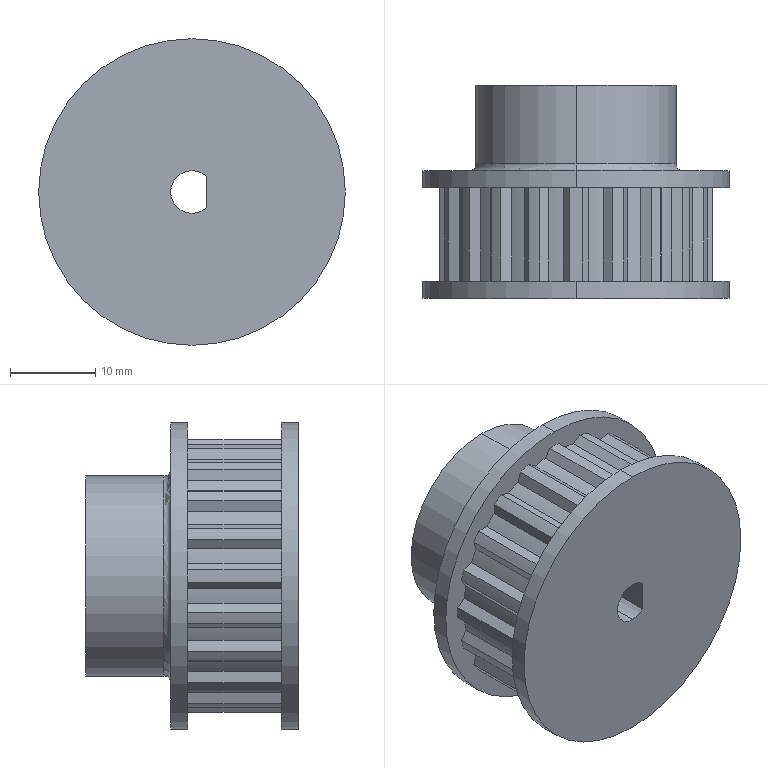Part | SolidWorks | features ICE 5, Extrusion 1, Fillet 1 | 1 solid | 98 faces | box 36 x 25 x 36 mm | volume 16244 mm3 | cylinder 50 | plane 46 | torus 2 | commonest cylinder face diameters 32 x21 30.016 x20 36 x4 5 x3 23.5 x2